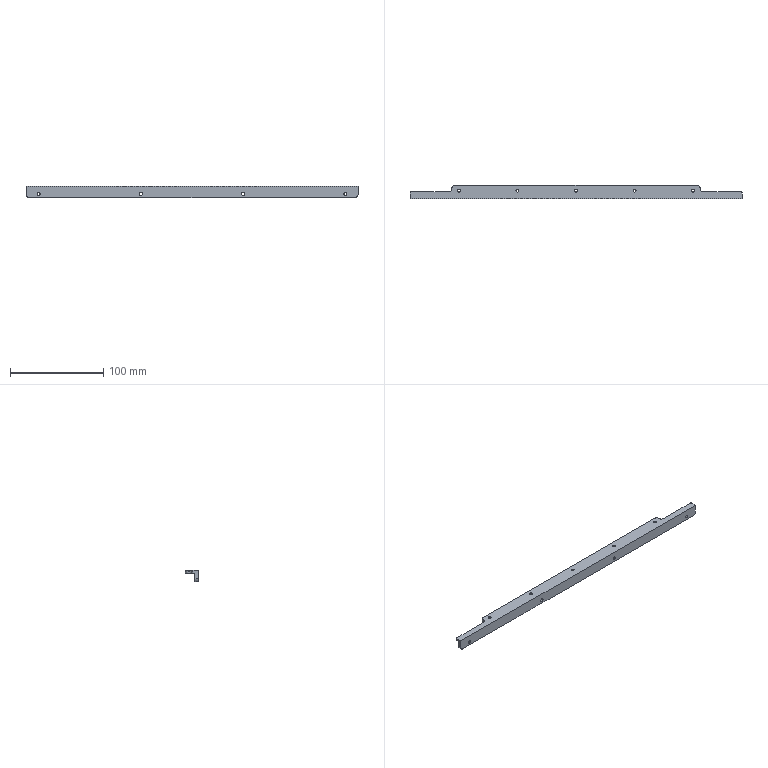NC program | NX | posted with a generic post | part box 356.96 x 14 x 12 mm
Lines 1 to 845 of 3585:
N10 G17 G21 G94 G90
(PLANAR_MILL , TOOL : D6开粗)
N12 T01 M6
N14 G54
N16 G17 G0 G90 X188.48 Y-5. B0. C0. S4500 M3
N18 G43 Z30. H1
N20 Z2.
N22 G94 G1 Z0. F800.
N24 X175.48
N26 X-175.48
N28 X-188.48
N30 Z2.
N32 G0 Z30.
(ADAPTIVE_MILLING , TOOL : D6开粗)
N34 X-181.367 Y-15.037 S6500
N36 Z-9.3
N38 G1 X-181.378 Y-14.888 Z-10.237 F3000.
N40 X-181.388 Y-14.738 Z-10.608
N42 X-181.399 Y-14.588 Z-10.88
N44 X-181.41 Y-14.439 Z-11.1
N46 X-181.421 Y-14.289 Z-11.284
N48 X-181.432 Y-14.14 Z-11.442
N50 X-181.443 Y-13.99 Z-11.58
N52 X-181.454 Y-13.84 Z-11.7
N54 X-181.464 Y-13.691 Z-11.805
N56 X-181.475 Y-13.541 Z-11.898
N58 X-181.486 Y-13.392 Z-11.979
N60 X-181.497 Y-13.242 Z-12.05
N62 X-181.508 Y-13.092 Z-12.11
N64 X-181.519 Y-12.943 Z-12.162
N66 X-181.529 Y-12.793 Z-12.205
N68 X-181.54 Y-12.644 Z-12.239
N70 X-181.551 Y-12.494 Z-12.266
N72 X-181.562 Y-12.344 Z-12.285
N74 X-181.573 Y-12.195 Z-12.296
N76 X-181.584 Y-12.045 Z-12.3
N78 X-181.657 Y-11.029
N80 G3 X-181.989 Y-10.531 R0.608
N82 G2 X-184.206 Y-8.065 R4.373
N84 X-184.894 Y-4.396 R11.849
N86 X-185. Y4.165 R173.128
N88 X-184.967 Y6.322 R23.537
N90 X-183.128 Y8.803 R3.678
N92 X-179.675 Y9.808 R8.418
N94 X-174.18 Y9.995 R58.875
N96 G1 X-169.93 Y10.
N98 X-131.864 Y10.001
N100 X-130.499 Y10.15
N102 X130.501
N104 G3 X136.267 Y10.003 R70.729
N106 G1 X139.011 Y10.
N108 X180.949 Y9.999
N110 G2 X183.56 Y8.492 R3.397
N112 X184.738 Y5.233 R7.218
N114 X184.99 Y-0.008 R41.644
N116 X184.984 Y-6.198 R589.03
N118 X183.287 Y-8.703 R3.571
N120 X179.985 Y-9.771 R7.794
N122 G1 X179.295 Y-10.043
N124 X178.479 Y-10.15
N126 X-178.543 Y-10.144
N128 G2 X-180.251 Y-9.991 R16.542
N130 X-183.265 Y-7.551 R4.627
N132 X-184.29 Y-3.775 R10.169
N134 X-184.495 Y2.344 R65.648
N136 X-184.457 Y4.842 R25.222
N138 X-182.037 Y8.184 R4.621
N140 X-178.273 Y9.27 R9.821
N142 X-172.467 Y9.493 R57.776
N144 G1 X-167.655 Y9.5
N146 X-133.304 Y9.502
N148 G3 X-132.852 Y9.682 R1.274
N150 G1 X-131.716 Y10.027
N152 G3 X-131.558 Y11.101 R0.6
N154 X-131.962 Y11.208 Z-12.264 R0.753
N156 G1 X-132.718 Y11.263 Z-12.2
N158 X-134.019 Y11.357 F15000.
N160 X-175.77
N162 G3 X-180.998 Y10.543 R17.721
N164 X-183.136 Y9.637 R14.582
N166 X-184.619 Y8.447 R5.326
N168 X-185.684 Y6.953 R7.067
N170 X-186.111 Y5.562 R4.113
N172 G1 X-186.352 Y3.468
N174 G3 X-186.367 Y-0.313 R22.035
N176 G1 X-186.064 Y-3.996
N178 G3 X-185.384 Y-7.226 R13.138
N180 X-184.177 Y-9.476 R8.753
N182 G1 X-183.48 Y-10.401
N184 G3 X-181.61 Y-11.641 R4.019
N186 G1 X-180.946 Y-11.852
N188 X-180.278 Y-12.051
N190 G3 X-179.942 Y-12.008 R0.62
N192 G1 X-178.984 Y-11.587
N194 X-178.609 Y-11.424 Z-12.235 F3000.
N196 X-178.238 Y-11.251 Z-12.269
N198 G3 X-178.006 Y-10.978 Z-12.3 R0.628
N200 X-178.481 Y-10.15 R0.6
N202 G1 X-179.295 Y-10.043
N204 G2 X-181.86 Y-8.185 R5.528
N206 X-183.561 Y-4.195 R8.781
N208 X-183.969 Y1.158 R33.24
N210 X-183.925 Y3.78 R19.191
N212 X-181.111 Y7.623 R5.252
N214 X-177.04 Y8.758 R10.996
N216 X-170.922 Y8.992 R62.
N218 G1 X-166.359 Y9.
N220 X-134.753
N222 G3 X-133.915 Y9.114 R1.715
N224 G1 X-133.089 Y9.556
N226 G3 X-132.882 Y10.433 R0.6
N228 X-133.423 Y10.693 Z-12.247 R0.67
N230 G1 X-133.979 Y10.749 Z-12.2
N232 X-135.392 Y10.886 F15000.
N234 X-173.079
N236 G3 X-177.488 Y10.557 R29.772
N238 G1 X-178.947 Y10.331
N240 G3 X-182.331 Y8.963 R9.047
N242 G1 X-183.026 Y8.458
N244 X-183.71 Y7.938
N246 G3 X-184.496 Y7.021 R3.856
N248 X-185.346 Y5.47 R17.7
N250 X-185.889 Y3.494 R6.037
N252 G1 X-185.904 Y3.201
N254 X-185.906 Y2.908
N256 X-185.856 Y0.939
N258 X-185.791 Y-1.03
N260 G3 X-185.124 Y-5.522 R26.068
N262 X-183.622 Y-8.869 R11.848
N264 G1 X-182.625 Y-10.416
N266 G3 X-182.16 Y-10.69 R0.603
N268 G1 X-181.162 Y-10.756
N270 X-180.763 Y-10.785 Z-12.234 F3000.
N272 X-180.364 Y-10.801 Z-12.268
N274 G3 X-180.019 Y-10.65 Z-12.3 R0.626
N276 X-180.055 Y-9.728 R0.6
N278 G1 X-180.707 Y-9.227
N280 G2 X-181.889 Y-7.281 R8.071
N282 X-183.267 Y-1.922 R15.481
N284 X-183.422 Y2.509 R31.124
N286 X-180.3 Y7.065 R5.669
N288 X-176.111 Y8.234 R11.687
N290 X-169.369 Y8.493 R65.346
N292 G1 X-165.244 Y8.499
N294 X-135.942 Y8.5
N296 G3 X-134.567 Y8.618 R5.649
N298 X-133.915 Y9.114 R3.309
N300 X-133.774 Y9.874 R0.6
N302 X-134.271 Y10.18 Z-12.249 R0.62
N304 G1 X-134.839 Y10.259 Z-12.2
N306 X-135.528 Y10.359 F15000.
N308 X-136.219 Y10.444
N310 X-172.428
N312 G3 X-176.819 Y10.01 R22.428
N314 X-178.973 Y9.509 R22.146
N316 X-181.317 Y8.626 R22.161
N318 X-183.369 Y6.996 R5.663
N320 G1 X-183.825 Y6.416
N322 X-184.253 Y5.815
N324 G3 X-185.205 Y3.517 R6.702
N326 X-185.281 Y2.35 R4.807
N328 G1 X-185.158 Y0.212
N330 X-185.021 Y-1.925
N332 G3 X-184.099 Y-6.797 R25.85
N334 G1 X-183.778 Y-7.886
N336 G3 X-183.564 Y-8.195 R0.613
N338 G1 X-182.706 Y-8.844
N340 X-182.38 Y-9.092 Z-12.235 F3000.
N342 X-182.048 Y-9.332 Z-12.269
N344 G3 X-181.697 Y-9.401 Z-12.3 R0.628
N346 X-181.208 Y-8.575 R0.6
N348 G2 X-181.66 Y-7.134 R4.882
N350 X-182.886 Y1.244 R30.586
N352 X-179.487 Y6.545 R6.
N354 X-175.103 Y7.732 R12.511
N356 X-168.423 Y7.991 R67.003
N358 G1 X-163.611 Y7.999
N360 X-137.065 Y8.
N362 G3 X-135.098 Y8.161 R7.568
N364 X-134.413 Y8.706 R5.592
N366 X-134.271 Y9.467 R0.6
N368 X-134.768 Y9.772 Z-12.249 R0.62
N370 G1 X-135.337 Y9.851 Z-12.2
N372 X-136.026 Y9.951 F15000.
N374 X-136.716 Y10.036
N376 X-170.339
N378 G3 X-175.47 Y9.574 R28.726
N380 G1 X-176.414 Y9.403
N382 X-177.357 Y9.222
N384 G3 X-180.393 Y8.107 R12.629
N386 X-181.917 Y7.074 R9.804
N388 G1 X-182.708 Y6.41
N390 G3 X-184.263 Y3.874 R5.503
N392 X-184.558 Y2.431 R9.246
N394 X-184.629 Y0.23 R9.68
N396 G1 X-184.493 Y-1.425
N398 X-184.327 Y-3.077
N400 X-184.1 Y-4.721
N402 X-183.843 Y-6.361
N404 X-183.802 Y-6.5
N406 X-183.732 Y-6.626
N408 X-183.058 Y-7.532
N410 X-182.812 Y-7.866 Z-12.235 F3000.
N412 X-182.558 Y-8.194 Z-12.27
N414 G3 X-182.252 Y-8.358 Z-12.3 R0.63
N416 X-181.539 Y-7.691 R0.6
N418 G2 X-181.646 Y-6.21 R9.717
N420 G1 X-182.177 Y-1.956
N422 G2 X-182.234 Y1.347 R13.815
N424 X-178.843 Y5.961 R6.211
N426 X-174.347 Y7.209 R12.722
N428 X-167.668 Y7.489 R64.51
N430 G1 X-162.856 Y7.499
N432 X-138.065 Y7.5
N434 G3 X-135.681 Y7.67 R11.107
N436 X-135.221 Y7.895 R1.019
N438 G1 X-134.864 Y8.329
N440 G3 X-134.797 Y8.989 R0.601
N442 X-135.273 Y9.31 Z-12.249 R0.621
N444 G1 X-135.847 Y9.419 Z-12.2
N446 X-137.112 Y9.657 F15000.
N448 X-167.096 Y9.659
N450 G3 X-173.708 Y9.154 R43.538
N452 G1 X-174.863 Y8.977
N454 X-176.017 Y8.79
N456 G3 X-179.056 Y7.853 R13.567
N458 X-180.92 Y6.698 R9.216
N460 G1 X-181.594 Y6.164
N462 X-182.258 Y5.618
N464 G3 X-183.153 Y4.412 R3.972
N466 X-183.578 Y3.317 R6.243
N468 G1 X-183.937 Y2.011
N470 G3 X-184.188 Y-0.878 R10.008
N472 G1 X-183.934 Y-5.17
N474 G3 X-183.801 Y-5.512 R0.614
N476 G1 X-183.118 Y-6.356
N478 X-182.877 Y-6.659 Z-12.233 F3000.
N480 X-182.626 Y-6.951 Z-12.265
N482 G3 X-182.252 Y-7.1 Z-12.3 R0.623
N484 X-181.63 Y-6.5 R0.6
N486 X-181.755 Y-0.879 R74.483
N488 G2 X-180.529 Y3.424 R6.752
N490 X-176.593 Y6.071 R7.725
N492 X-171.481 Y6.871 R20.513
N494 X-161.671 Y6.999 R206.807
N496 G1 X-139.063 Y7.
N498 G3 X-136.204 Y7.183 R15.03
N500 X-135.586 Y7.45 R1.238
N502 G1 X-135.189 Y7.933
N504 G3 X-135.132 Y8.612 R0.601
N506 X-135.65 Y8.924 Z-12.247 R0.667
N508 G1 X-136.193 Y9.027 Z-12.2
N510 X-137.437 Y9.261 F15000.
N512 X-163.357 Y9.263
N514 G3 X-172.185 Y8.677 R66.864
N516 G1 X-173.712 Y8.476
N518 X-175.237 Y8.263
N520 G3 X-178.25 Y7.416 R14.269
N522 G1 X-179.178 Y7.031
N524 G3 X-180.703 Y5.957 R5.471
N526 X-182.117 Y4.261 R12.322
N528 G1 X-182.676 Y3.456
N530 X-183.224 Y2.643
N532 G3 X-183.759 Y-0.078 R4.076
N534 G1 X-183.5 Y-1.735
N536 X-183.113 Y-2.852
N538 X-182.768 Y-3.828 Z-12.288 F3000.
N540 X-182.687 Y-3.951 Z-12.3
N542 G3 X-181.63 Y-3.563 R0.6
N544 G1 Y-0.999
N546 X-181.526 Y-0.077
N548 G2 X-179.682 Y3.285 R8.632
N550 X-175.36 Y5.716 R8.959
N552 X-169.976 Y6.401 R25.27
N554 X-160.477 Y6.498 R270.598
N556 G1 X-139.876 Y6.5
N558 G3 X-136.637 Y6.708 R17.175
N560 X-135.821 Y7.064 R1.561
N562 G1 X-135.573 Y7.466
N564 G3 X-135.516 Y8.145 R0.601
N566 X-136.033 Y8.457 Z-12.247 R0.667
N568 G1 X-136.577 Y8.56 Z-12.2
N570 X-137.821 Y8.794 F15000.
N572 X-160.415 Y8.796
N574 G3 X-169.995 Y8.293 R91.63
N576 G1 X-171.726 Y8.114
N578 X-173.457 Y7.921
N580 G3 X-177.52 Y6.881 R18.008
N582 X-179.598 Y5.764 R10.798
N584 G1 X-180.369 Y5.225
N586 G3 X-181.406 Y4.117 R4.744
N588 G1 X-181.683 Y3.71
N590 X-181.95 Y3.296
N592 X-182.001 Y3.133
N594 X-182.177 Y2.064
N596 X-182.324 Y1.141 Z-12.279 F3000.
N598 X-182.312 Y1.018 Z-12.29
N600 X-182.28 Y0.899 Z-12.3
N602 G3 X-181.219 Y0.801 R0.6
N604 G1 X-180.725 Y1.587
N606 G2 X-177.208 Y4.313 R12.849
N608 X-172.1 Y5.686 R15.287
N610 X-164.985 Y5.986 R70.056
N612 G1 X-159.485 Y5.998
N614 X-140.873 Y5.999
N616 G3 X-137.254 Y6.191 R22.944
N618 X-136.085 Y6.611 R2.72
N620 X-135.736 Y7.187 R2.348
N622 X-135.836 Y7.889 R0.601
N624 X-136.382 Y8.061 Z-12.25 R0.622
N626 G1 X-136.966 Y8.004 Z-12.2
N628 X-138.306 Y7.876 F15000.
N630 X-166.016
N632 G3 X-172.519 Y7.45 R52.331
N634 X-176.655 Y6.505 R23.275
N636 X-178.689 Y5.63 R14.434
N638 G1 X-180.067 Y4.905
N640 G3 X-180.351 Y4.582 R0.608
N642 G1 X-180.716 Y3.592
N644 X-180.853 Y3.23 Z-12.233 F3000.
N646 X-180.977 Y2.862 Z-12.266
N648 G3 X-180.915 Y2.468 Z-12.3 R0.623
N650 X-180.067 Y2.245 R0.6
N652 G2 X-178.129 Y3.298 R13.035
N654 X-171.057 Y5.229 R19.06
N656 X-162.626 Y5.493 R97.412
N658 G1 X-159.189 Y5.498
N660 X-141.378 Y5.5
N662 G3 X-137.488 Y5.742 R21.85
N664 X-136.288 Y6.209 R2.628
N666 X-135.945 Y6.796 R4.354
N668 X-136.068 Y7.52 R0.601
N670 X-136.632 Y7.661 Z-12.249 R0.621
N672 G1 X-137.201 Y7.564 Z-12.2
N674 X-138.194 Y7.398 F15000.
N676 X-178.678 Y4.987
N678 G3 X-179.117 Y4.755 R0.604
N680 G1 X-179.524 Y4.228
N682 X-179.77 Y3.914 Z-12.234 F3000.
N684 X-180.006 Y3.592 Z-12.268
N686 G3 X-180.073 Y3.22 Z-12.3 R0.626
N688 X-179.281 Y2.739 R0.6
N690 G2 X-177.481 Y3.266 R12.828
N692 X-171.568 Y4.62 R32.819
N694 X-163.768 Y4.983 R72.376
N696 G1 X-158.268 Y4.998
N698 X-142.373 Y4.999
N700 G3 X-138.107 Y5.214 R28.899
N702 X-136.459 Y5.798 R3.751
N704 X-136.181 Y6.355 R1.001
N706 G1 X-136.152 Y6.41
N708 G3 X-136.216 Y7.131 R0.661
N710 X-136.889 Y7.372 Z-12.237 R0.709
N712 G1 X-137.32 Y7.341 Z-12.2
N714 X-174.812 Y4.629 F15000.
N716 X-175.991 Y4.543 Z-12.3 F3000.
N718 X-178.525 Y4.36
N720 G3 X-178.403 Y3.046 R-0.66
N722 X-176.246 Y3.281 R52.797
N724 G2 X-170.316 Y4.211 R57.736
N726 X-160.885 Y4.494 R114.394
N728 G1 X-157.198 Y4.497
N730 X-142.876 Y4.499
N732 G3 X-138.389 Y4.744 R28.946
N734 X-136.584 Y5.406 R4.172
N736 X-136.26 Y6.095 R1.325
N738 X-136.412 Y6.741 R0.661
N740 X-137.042 Y6.939 Z-12.242 R0.718
N742 G1 X-137.536 Y6.909 Z-12.2
N744 X-174.787 Y4.628 F15000.
N746 X-175.967 Y4.556 Z-12.3 F3000.
N748 X-177.394 Y4.469
N750 G3 X-177.354 Y3.15 R0.66
N752 X-172.591 Y3.451 R26.394
N754 G2 X-162.486 Y3.981 R85.748
N756 G1 X-152.486 Y3.998
N758 G3 X-141.201 Y4.038 R573.417
N760 X-137.754 Y4.491 R13.682
N762 X-136.6 Y5.117 R2.63
N764 X-136.381 Y5.698 R1.892
N766 X-136.541 Y6.352 R0.661
N768 X-137.161 Y6.542 Z-12.243 R0.728
N770 G1 X-137.669 Y6.515 Z-12.2
N772 X-172.626 Y4.628 F15000.
N774 X-173.807 Y4.565 Z-12.3 F3000.
N776 X-175.577 Y4.469
N778 G3 X-175.542 Y3.15 R0.66
N780 X-167.998 Y3.339 R90.168
N782 G2 X-155. Y3.497 R310.755
N784 G3 X-141.818 Y3.536 R788.653
N786 X-138.095 Y3.994 R15.721
N788 X-136.656 Y4.773 R2.943
N790 X-136.495 Y5.321 R2.028
N792 X-136.655 Y5.974 R0.661
N794 X-137.272 Y6.166 Z-12.243 R0.729
N796 G1 X-137.783 Y6.141 Z-12.2
N798 X-168.699 Y4.628 F15000.
N800 X-169.879 Y4.57 Z-12.3 F3000.
N802 X-171.949 Y4.469
N804 G3 X-171.917 Y3.15 R0.66
N806 G1 X-141.115 Y3.153
N808 G3 X-137.713 Y3.745 R9.96
N810 X-136.642 Y4.515 R2.137
N812 X-136.545 Y5.065 R1.702
N814 X-136.822 Y5.67 R0.661
N816 X-137.515 Y5.722 Z-12.239 R0.721
N818 G1 X-137.948 Y5.58 Z-12.2
N820 X-140.845 Y4.631 F15000.
N822 X-141.521 Y4.402 Z-12.261 F3000.
N824 G3 X-141.836 Y4.069 Z-12.3 R0.68
N826 X-141.229 Y3.15 R0.66
N828 X-138.739 Y3.178 R36.948
N830 X-136.776 Y4.03 R3.27
N832 X-136.577 Y4.736 R1.141
N834 X-136.922 Y5.383 R0.661
N836 X-137.638 Y5.334 Z-12.236 R0.708
N838 G1 X-138.016 Y5.134 Z-12.2
N840 X-138.964 Y4.631 F15000.
N842 X-139.495 Y4.342 Z-12.251 F3000.
N844 G3 X-139.763 Y3.852 Z-12.3 R0.67
N846 X-139.104 Y3.15 R0.66
N848 X-137.684 Y3.243 R5.063
N850 X-136.695 Y3.912 R1.581
N852 X-136.611 Y4.392 R1.983
N854 X-136.99 Y5.056 R0.661
N856 X-137.683 Y4.973 Z-12.238 R0.675
N858 G1 X-138.055 Y4.723 Z-12.2
N860 X-138.189 Y4.633 F15000.
N862 X-138.675 Y4.297 Z-12.25 F3000.
N864 G3 X-138.888 Y3.766 Z-12.3 R0.67
N866 X-138.229 Y3.15 R0.66
N868 X-136.928 Y3.444 R1.97
N870 X-136.638 Y4.125 R0.807
N872 X-137.729 Y4.687 R0.66
N874 G1 X-137.988 Y4.464
N876 X-138.238 Y4.231
N878 G3 X-137.729 Y3.15 R0.66
N880 X-136.782 Y3.46 R1.072
N882 X-136.65 Y3.957 R0.799
N884 X-138.207 Y3.855 R-0.782
N886 X-137.417 Y3.15 R0.796
N888 X-136.663 Y3.731 R0.676
N890 X-137.112 Y4.397 R0.606
N892 G1 X-138.069 Y4.646
N894 X-138.215 Y4.684 Z-12.296
N896 X-138.36 Y4.721 Z-12.285
N898 X-138.505 Y4.759 Z-12.266
N900 X-138.65 Y4.797 Z-12.239
N902 X-138.795 Y4.835 Z-12.205
N904 X-138.94 Y4.873 Z-12.162
N906 X-139.086 Y4.91 Z-12.11
N908 X-139.231 Y4.948 Z-12.05
N910 X-139.376 Y4.986 Z-11.979
N912 X-139.521 Y5.024 Z-11.898
N914 X-139.666 Y5.062 Z-11.805
N916 X-139.811 Y5.099 Z-11.7
N918 X-139.957 Y5.137 Z-11.58
N920 X-140.102 Y5.175 Z-11.442
N922 X-140.247 Y5.213 Z-11.284
N924 X-140.392 Y5.251 Z-11.1
N926 X-140.537 Y5.288 Z-10.88
N928 X-140.682 Y5.326 Z-10.608
N930 X-140.828 Y5.364 Z-10.237
N932 X-140.973 Y5.402 Z-9.3
N934 G0 Z30.
N936 X133.35 Y11.628
N938 Z-9.3
N940 G1 X133.2 Z-10.237
N942 X133.05 Z-10.608
N944 X132.9 Z-10.88
N946 X132.75 Z-11.1
N948 X132.6 Z-11.284
N950 X132.45 Z-11.442
N952 X132.3 Z-11.58
N954 X132.15 Z-11.7
N956 X132. Z-11.805
N958 X131.85 Z-11.898
N960 X131.7 Z-11.979
N962 X131.55 Z-12.05
N964 X131.4 Z-12.11
N966 X131.25 Z-12.162
N968 X131.1 Z-12.205
N970 X130.95 Z-12.239
N972 X130.8 Z-12.266
N974 X130.65 Z-12.285
N976 X130.5 Z-12.296
N978 X130.35 Z-12.3
N980 G3 X130.069 Y10.485 R0.606
N982 X130.874 Y10.113 R3.541
N984 G2 X132.297 Y9.856 R4.726
N986 G3 X135.885 Y9.541 R19.417
N988 X142.949 Y9.5 R595.839
N990 G1 X179.349 Y9.498
N992 G2 X183.057 Y7.251 R4.494
N994 X184.239 Y3.52 R9.188
N996 X184.492 Y-2.409 R52.47
N998 X184.456 Y-4.844 R23.974
N1000 X182.036 Y-8.185 R4.625
N1002 G1 X181.159 Y-8.661
N1004 X180.707 Y-9.227
N1006 X180.055 Y-9.728
N1008 X179.882 Y-9.8
N1010 G3 X179.904 Y-10.917 R0.6
N1012 X180.323 Y-10.927 Z-12.264 R0.751
N1014 G1 X181.07 Y-10.805 Z-12.2
N1016 X181.654 Y-10.712 F15000.
N1018 X182.236 Y-10.608
N1020 X182.349 Y-10.557
N1022 X182.451 Y-10.488
N1024 X183.403 Y-9.67
N1026 X184.346 Y-8.84
N1028 G3 X185.933 Y-6.316 R6.003
N1030 X186.268 Y-4.883 R9.256
N1032 X186.408 Y-2.687 R9.947
N1034 G1 X186.281 Y0.069
N1036 X186.138 Y2.823
N1038 G3 X185.331 Y6.742 R16.956
N1040 X183.851 Y9.199 R5.954
N1042 X182.356 Y10.422 R7.193
N1044 X179.692 Y11.201 R5.295
N1046 G1 X134.061 Y11.767
N1048 X133.94 Y11.754
N1050 X133.823 Y11.721
N1052 X132.748 Y11.274
N1054 X132.388 Y11.128 Z-12.233 F3000.
N1056 X132.034 Y10.968 Z-12.266
N1058 G3 X131.787 Y10.657 Z-12.3 R0.624
N1060 X132.18 Y9.886 R0.6
N1062 X133.702 Y9.399 R67.688
N1064 X137.637 Y9.045 R21.558
N1066 X143.824 Y9. R577.308
N1068 G1 X177.911 Y8.998
N1070 G2 X182.627 Y6.108 R5.249
N1072 X183.759 Y2.036 R11.026
N1074 X183.945 Y-3.581 R38.314
N1076 X182.269 Y-6.861 R5.317
N1078 G3 X181.577 Y-7.612 R4.027
N1080 G2 X181.208 Y-8.575 R7.666
N1082 G1 X181.094 Y-8.724
N1084 G3 X181.732 Y-9.667 R0.6
N1086 X182.095 Y-9.426 Z-12.263 R0.937
N1088 G1 X182.652 Y-8.936 Z-12.2
N1090 X183.598 Y-8.103 F15000.
N1092 G3 X184.487 Y-6.995 R12.763
N1094 G1 X184.72 Y-6.621
N1096 X184.928 Y-6.232
N1098 X185.218 Y-5.638
N1100 X185.48 Y-5.031
N1102 G3 X185.85 Y-2.723 R6.052
N1104 G1 X185.785 Y-0.798
N1106 X185.706 Y1.126
N1108 G3 X185.236 Y4.244 R18.563
N1110 G1 X185.078 Y4.909
N1112 X184.89 Y5.566
N1114 G3 X183.971 Y7.343 R7.292
N1116 X182.677 Y8.969 R13.087
N1118 X180.887 Y10.182 R5.836
N1120 X178.206 Y10.799 R6.276
N1122 G1 X135.096 Y11.008
N1124 X133.778 Y10.877
N1126 X133.38 Y10.84 Z-12.234 F3000.
N1128 X132.984 Y10.79 Z-12.268
N1130 G3 X132.668 Y10.584 Z-12.3 R0.626
N1132 X132.855 Y9.681 R0.6
N1134 X135.827 Y8.743 R6.723
N1136 X142.208 Y8.506 R62.634
N1138 G1 X145.449 Y8.5
N1140 X176.599 Y8.499
N1142 G2 X180.549 Y7.206 R5.902
N1144 X182.778 Y3.515 R7.31
N1146 X183.39 Y-2.618 R21.021
N1148 X182.218 Y-5.686 R6.665
N1150 G3 X181.653 Y-6.642 R7.038
N1152 G1 X181.524 Y-7.807
N1154 G3 X182.251 Y-8.47 R0.6
N1156 X182.676 Y-8.134 Z-12.253 R0.683
N1158 G1 X183.033 Y-7.622 Z-12.2
N1160 X183.828 Y-6.476 F15000.
N1162 X184.273 Y-5.714
N1164 X184.707 Y-4.946
N1166 G3 X185.289 Y-2.445 R5.335
N1168 G1 X185.254 Y-0.475
N1170 G3 X184.23 Y4.811 R17.486
N1172 X182.244 Y8.18 R11.059
N1174 X179.639 Y9.862 R6.215
N1176 X176.578 Y10.344 R10.187
N1178 G1 X135.811 Y10.625
N1180 X134.494 Y10.494
N1182 X134.096 Y10.457 Z-12.234 F3000.
N1184 X133.7 Y10.407 Z-12.268
N1186 G3 X133.384 Y10.2 Z-12.3 R0.626
N1188 X133.571 Y9.298 R0.6
N1190 X134.619 Y8.735 R11.114
N1192 X137.885 Y8.154 R11.928
N1194 X145.699 Y8.001 R125.793
N1196 G1 X175.161 Y8.
N1198 G2 X178.296 Y7.551 R8.349
N1200 X181.754 Y4.078 R6.399
N1202 X182.779 Y-1.908 R13.701
N1204 X181.818 Y-5.036 R9.517
N1206 G3 X181.63 Y-5.562 R3.178
N1208 G1 Y-6.812
N1210 G3 X182.245 Y-7.412 R0.6
N1212 X182.741 Y-7.132 Z-12.25 R0.622
N1214 G1 X183.101 Y-6.664 Z-12.2
N1216 X183.492 Y-6.164 F15000.
N1218 X183.871 Y-5.654
N1220 X183.934 Y-5.482
N1222 X184.294 Y-3.698
N1224 X184.641 Y-1.912
N1226 G3 X184.618 Y0.405 R7.582
N1228 X184.266 Y2.14 R16.237
N1230 G1 X183.87 Y3.616
N1232 G3 X182.882 Y5.928 R11.453
N1234 G1 X182.392 Y6.78
N1236 G3 X181.132 Y8.059 R4.683
N1238 G1 X180.762 Y8.299
N1240 X180.377 Y8.515
N1242 X179.722 Y8.85
N1244 X179.053 Y9.153
N1246 G3 X176.919 Y9.648 R6.89
N1248 X173.232 Y9.813 R70.125
N1250 G1 X136.27 Y10.403
N1252 X136.178 Y10.397
N1254 X134.916 Y10.222
N1256 X134.179 Y10.113 Z-12.263 F3000.
N1258 G3 X133.838 Y9.854 Z-12.3 R0.618
N1260 X133.966 Y9.073 R0.6
N1262 X136.13 Y8.02 R4.355
N1264 X140.714 Y7.566 R25.051
N1266 X148.636 Y7.5 R362.047
N1268 G1 X174.349 Y7.499
N1270 G2 X177.662 Y6.983 R8.7
N1272 X181.241 Y3.304 R6.717
N1274 X182.134 Y-0.762 R10.91
N1276 G1 X182.127 Y-3.224
N1278 X181.641 Y-4.355
N1280 X181.63 Y-5.614
N1282 G3 X182.216 Y-6.214 R0.6
N1284 X182.729 Y-5.952 Z-12.249 R0.621
N1286 G1 X183.101 Y-5.503 Z-12.2
N1288 X183.795 Y-4.667 F15000.
N1290 G3 X183.934 Y-4.284 R0.609
N1292 G1 X183.937 Y-2.56
N1294 X183.926 Y-0.837
N1296 G3 X183.419 Y2.68 R15.999
N1298 X182.488 Y4.829 R9.492
N1300 X181.054 Y6.782 R10.329
N1302 G1 X180.659 Y7.166
N1304 X180.242 Y7.526
N1306 X179.47 Y8.136
N1308 G3 X178.366 Y8.657 R3.442
N1310 G1 X177.653 Y8.845
N1312 X176.934 Y9.006
N1314 G3 X175.473 Y9.176 R10.761
N1316 X169.939 Y9.371 R204.653
N1318 G1 X136.705 Y10.046
N1320 X136.61 Y10.04
N1322 X135.35 Y9.865
N1324 X134.613 Y9.756 Z-12.263 F3000.
N1326 G3 X134.273 Y9.497 Z-12.3 R0.618
N1328 X134.401 Y8.716 R0.6
N1330 X136.854 Y7.53 R4.838
N1332 X141.832 Y7.062 R27.927
N1334 X148.886 Y7.001 R437.195
N1336 G1 X173.286 Y6.999
N1338 G2 X176.679 Y6.563 R10.269
N1340 X180.616 Y2.823 R6.832
N1342 X181.325 Y0.497 R9.483
N1344 G1 X181.526 Y-0.077
N1346 X181.63 Y-1.001
N1348 Y-4.438
N1350 G3 X182.648 Y-4.869 R0.6
N1352 X182.833 Y-4.536 Z-12.267 R0.778
N1354 G1 X183.104 Y-3.786 Z-12.2
N1356 X183.475 Y-2.762 F15000.
N1358 X183.5 Y-2.661
N1360 X183.511 Y-2.557
N1362 X183.504 Y-1.081
N1364 G3 X182.583 Y2.837 R10.597
N1366 G1 X182.283 Y3.51
N1368 X181.954 Y4.17
N1370 G3 X181.138 Y5.387 R8.715
N1372 G1 X180.675 Y5.962
N1374 X180.191 Y6.519
N1376 G3 X179.628 Y6.989 R3.259
N1378 G1 X178.697 Y7.587
N1380 G3 X175.945 Y8.55 R7.953
N1382 G1 X175.399 Y8.62
N1384 X174.85 Y8.659
N1386 X169.866 Y8.843
N1388 X164.882 Y8.99
N1390 X137.089 Y9.676
N1392 X135.855 Y9.443
N1394 X135.477 Y9.373 Z-12.233 F3000.
N1396 X135.101 Y9.289 Z-12.265
N1398 G3 X134.793 Y9.027 Z-12.3 R0.623
N1400 X134.85 Y8.348 R0.601
N1402 X136.359 Y7.365 R3.063
N1404 X140.261 Y6.68 R15.11
N1406 X149.012 Y6.501 R136.692
N1408 G1 X171.974
N1410 G2 X175.451 Y6.205 R14.15
N1412 X180.003 Y2.322 R6.909
N1414 G1 X180.725 Y1.587
N1416 X181.219 Y0.801
N1418 X181.343 Y0.447
N1420 G3 X182.507 Y0.693 R0.6
N1422 G1 X182.295 Y1.856 Z-12.2
N1424 X182.102 Y2.871 F15000.
N1426 X182.031 Y3.016
N1428 X181.206 Y4.239
N1430 G3 X179.965 Y5.588 R8.305
N1432 G1 X178.902 Y6.503
N1434 G3 X176.563 Y7.712 R6.73
N1436 X174.038 Y8.163 R9.873
N1438 G1 X164.071 Y8.558
N1440 X159.641 Y8.722
N1442 X137.312 Y9.484
N1444 X137.178 Y9.474
N1446 X136.038 Y9.255
N1448 X135.65 Y9.183 Z-12.233 F3000.
N1450 X135.264 Y9.098 Z-12.267
N1452 G3 X134.965 Y8.855 Z-12.3 R0.625
N1454 X135.008 Y8.154 R0.601
N1456 X136.836 Y6.899 R3.517
N1458 X140.888 Y6.19 R16.076
N1460 X149.201 Y6.002 R126.532
N1462 G1 X171.098 Y6.001
N1464 G2 X174.642 Y5.723 R15.644
N1466 X178.634 Y3.133 R7.161
N1468 G3 X179.281 Y2.739 R1.042
N1470 G1 X180.112 Y2.2
N1472 G3 X181.097 Y2.413 R0.6
N1474 X181.042 Y2.966 Z-12.252 R0.673
N1476 G1 X180.799 Y3.523 Z-12.2
N1478 X180.549 Y4.103 F15000.
N1480 X180.289 Y4.677
N1482 X180.209 Y4.777
N1484 X180.112 Y4.861
N1486 X178.906 Y5.668
N1488 X177.693 Y6.465
N1490 G3 X175.971 Y7.203 R6.894
N1492 X172.939 Y7.806 R20.313
N1494 G1 X172.278 Y7.862
N1496 X171.616 Y7.89
N1498 X137.855 Y8.505
N1500 X136.487 Y8.697
N1502 X135.748 Y8.797 Z-12.263 F3000.
N1504 G3 X135.349 Y8.644 Z-12.3 R0.619
N1506 X135.286 Y7.816 R0.6
N1508 X137.224 Y6.454 R3.742
N1510 X141.455 Y5.701 R16.553
N1512 X150.762 Y5.502 R139.79
N1514 G1 X170.161 Y5.501
N1516 G2 X173.833 Y5.244 R17.888
N1518 X177.312 Y3.48 R7.997
N1520 G3 X178.403 Y3.046 R1.477
N1522 G1 X178.993 Y2.84
N1524 G3 X179.782 Y3.299 R0.6
N1526 X179.596 Y3.864 Z-12.248 R0.673
N1528 G1 X179.248 Y4.309 Z-12.2
N1530 X179.006 Y4.625 F15000.
N1532 X178.753 Y4.932
N1534 G3 X178.391 Y5.088 R0.61
N1536 G1 X137.806 Y8.025
N1538 X136.885 Y8.181
N1540 X136.156 Y8.298 Z-12.263 F3000.
N1542 G3 X135.749 Y8.15 Z-12.3 R0.618
N1544 X135.614 Y7.415 R0.601
N1546 X136.797 Y6.35 R2.562
N1548 X140.244 Y5.393 R10.707
N1550 X146.854 Y5.028 R57.123
N1552 G1 X152.324 Y5.001
N1554 X169.598 Y5.
N1556 G2 X173.328 Y4.701 R16.828
N1558 X176.353 Y3.386 R10.77
N1560 G3 X176.918 Y3.15 R1.709
N1562 G2 X177.978 Y3.094 R6.349
N1564 G3 X178.112 Y4.407 R-0.66
N1566 G1 X176.883 Y4.519
N1568 X175.706 Y4.627 Z-12.2
N1570 X136.893 Y8.168 F15000.
N1572 X136.567 Y8.2 Z-12.228 F3000.
N1574 X136.239 Y8.22 Z-12.256
N1576 G3 X135.782 Y7.988 Z-12.3 R0.677
N1578 X135.703 Y7.25 R0.661
N1580 X137.002 Y5.961 R2.755
N1582 X140.407 Y4.951 R10.526
N1584 X146.864 Y4.539 R51.252
N1586 G1 X153.824 Y4.501
N1588 X168.786 Y4.5
N1590 G2 X172.764 Y4.177 R17.71
N1592 X175.494 Y3.189 R16.722
N1594 G1 X175.676 Y3.15
N1596 X176.926
N1598 G3 X176.982 Y4.468 R0.66
N1600 G1 X176.276 Y4.527
N1602 X175.098 Y4.627 Z-12.2
N1604 X137.074 Y7.841 F15000.
N1606 X136.744 Y7.87 Z-12.228 F3000.
N1608 X136.413 Y7.889 Z-12.256
N1610 G3 X135.961 Y7.661 Z-12.3 R0.677
N1612 X135.879 Y6.919 R0.661
N1614 X137.296 Y5.512 R2.955
N1616 X140.886 Y4.459 R11.165
N1618 X147.861 Y4.035 R55.119
N1620 G1 X155.074 Y4.002
N1622 X172.7 Y3.994
N1624 G2 X173.922 Y3.396 R13.417
N1626 G3 X174.562 Y3.15 R2.474
N1628 G1 X175.687
N1630 G3 X175.738 Y4.468 R0.66
N1632 G1 X174.873 Y4.535
N1634 X173.694 Y4.627 Z-12.2
N1636 X137.278 Y7.459 F15000.
N1638 X136.947 Y7.486 Z-12.228 F3000.
N1640 X136.615 Y7.502 Z-12.256
N1642 G3 X136.166 Y7.273 Z-12.3 R0.677
N1644 X136.085 Y6.533 R0.661
N1646 X137.512 Y5.096 R2.994
N1648 X141.167 Y3.993 R11.266
N1650 X147.931 Y3.546 R52.165
N1652 X157.386 Y3.502 R677.74
N1654 G1 X171.575 Y3.495
N1656 X172.857 Y3.15
N1658 X174.607
N1660 G3 X174.654 Y4.468 R0.66
N1662 G1 X173.639 Y4.542
N1664 X172.46 Y4.627 Z-12.2
N1666 X137.438 Y7.16 F15000.
N1668 X137.1 Y7.186 Z-12.229 F3000.
N1670 X136.761 Y7.201 Z-12.257
N1672 G3 X136.321 Y6.982 Z-12.3 R0.678
N1674 X136.182 Y6.352 R0.662
N1676 X137.143 Y5.042 R2.318
N1678 X140.242 Y3.758 R8.36
N1680 X145.332 Y3.15 R30.388
N1682 G1 X172.895